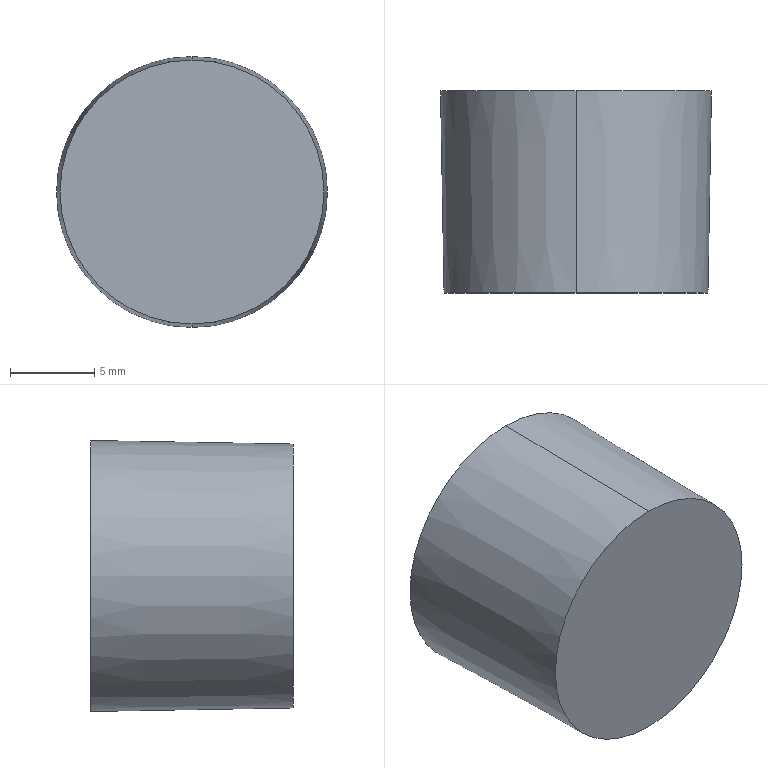Part | STEP file | 4-20.sldasm-Part-339 | 1 solid | 4 faces | box 16.088 x 12 x 16.088 mm | volume 2376 mm3 | cone 2 | plane 2
STEP:
#1=CARTESIAN_POINT('',(50.,-12.,82.165));
#2=VERTEX_POINT('',#1);
#3=CARTESIAN_POINT('',(50.,-12.,97.835));
#4=VERTEX_POINT('',#3);
#5=CARTESIAN_POINT('',(50.,-12.,90.));
#6=DIRECTION('',(0.,1.,0.));
#7=DIRECTION('',(0.,0.,-1.));
#8=AXIS2_PLACEMENT_3D('',#5,#6,#7);
#9=CIRCLE('',#8,7.835);
#10=EDGE_CURVE('',#2,#4,#9,.T.);
#11=ORIENTED_EDGE('',*,*,#10,.T.);
#12=CARTESIAN_POINT('',(50.,0.,98.044));
#13=VERTEX_POINT('',#12);
#14=CARTESIAN_POINT('',(50.,-28.035,97.555));
#15=DIRECTION('',(0.,0.9998,0.01745));
#16=VECTOR('',#15,1000.);
#17=LINE('',#14,#16);
#18=EDGE_CURVE('',#4,#13,#17,.T.);
#19=ORIENTED_EDGE('',*,*,#18,.T.);
#20=CARTESIAN_POINT('',(50.,0.,81.956));
#21=VERTEX_POINT('',#20);
#22=CARTESIAN_POINT('',(50.,0.,90.));
#23=DIRECTION('',(0.,1.,0.));
#24=DIRECTION('',(0.,0.,-1.));
#25=AXIS2_PLACEMENT_3D('',#22,#23,#24);
#26=CIRCLE('',#25,8.044);
#27=EDGE_CURVE('',#21,#13,#26,.T.);
#28=ORIENTED_EDGE('',*,*,#27,.F.);
#29=CARTESIAN_POINT('',(50.,-28.035,82.445));
#30=DIRECTION('',(0.,0.9998,-0.01745));
#31=VECTOR('',#30,1000.);
#32=LINE('',#29,#31);
#33=EDGE_CURVE('',#2,#21,#32,.T.);
#34=ORIENTED_EDGE('',*,*,#33,.F.);
#35=EDGE_LOOP('',(#11,#19,#28,#34));
#36=FACE_OUTER_BOUND('',#35,.T.);
#37=CARTESIAN_POINT('',(50.,-28.035,90.));
#38=DIRECTION('',(0.,1.,0.));
#39=DIRECTION('',(0.,0.,-1.));
#40=AXIS2_PLACEMENT_3D('',#37,#38,#39);
#41=CONICAL_SURFACE('',#40,7.555,0.01745);
#42=ADVANCED_FACE('',(#36),#41,.T.);
#43=ORIENTED_EDGE('',*,*,#10,.F.);
#44=CARTESIAN_POINT('',(50.,-12.,90.));
#45=DIRECTION('',(0.,1.,0.));
#46=DIRECTION('',(0.,0.,-1.));
#47=AXIS2_PLACEMENT_3D('',#44,#45,#46);
#48=CIRCLE('',#47,7.835);
#49=EDGE_CURVE('',#4,#2,#48,.T.);
#50=ORIENTED_EDGE('',*,*,#49,.F.);
#51=EDGE_LOOP('',(#43,#50));
#52=FACE_OUTER_BOUND('',#51,.T.);
#53=CARTESIAN_POINT('',(50.,-12.,81.956));
#54=DIRECTION('',(0.,-1.,0.));
#55=DIRECTION('',(0.,0.,1.));
#56=AXIS2_PLACEMENT_3D('',#53,#54,#55);
#57=PLANE('',#56);
#58=ADVANCED_FACE('',(#52),#57,.T.);
#59=ORIENTED_EDGE('',*,*,#18,.F.);
#60=ORIENTED_EDGE('',*,*,#49,.T.);
#61=ORIENTED_EDGE('',*,*,#33,.T.);
#62=CARTESIAN_POINT('',(50.,0.,90.));
#63=DIRECTION('',(0.,1.,0.));
#64=DIRECTION('',(0.,0.,-1.));
#65=AXIS2_PLACEMENT_3D('',#62,#63,#64);
#66=CIRCLE('',#65,8.044);
#67=EDGE_CURVE('',#13,#21,#66,.T.);
#68=ORIENTED_EDGE('',*,*,#67,.F.);
#69=EDGE_LOOP('',(#59,#60,#61,#68));
#70=FACE_OUTER_BOUND('',#69,.T.);
#71=CARTESIAN_POINT('',(50.,-28.035,90.));
#72=DIRECTION('',(0.,1.,0.));
#73=DIRECTION('',(0.,0.,-1.));
#74=AXIS2_PLACEMENT_3D('',#71,#72,#73);
#75=CONICAL_SURFACE('',#74,7.555,0.01745);
#76=ADVANCED_FACE('',(#70),#75,.T.);
#77=ORIENTED_EDGE('',*,*,#27,.T.);
#78=ORIENTED_EDGE('',*,*,#67,.T.);
#79=EDGE_LOOP('',(#77,#78));
#80=FACE_OUTER_BOUND('',#79,.T.);
#81=CARTESIAN_POINT('',(50.,0.,81.956));
#82=DIRECTION('',(0.,1.,0.));
#83=DIRECTION('',(0.,0.,-1.));
#84=AXIS2_PLACEMENT_3D('',#81,#82,#83);
#85=PLANE('',#84);
#86=ADVANCED_FACE('',(#80),#85,.T.);
#87=CLOSED_SHELL('',(#42,#58,#76,#86));
#88=MANIFOLD_SOLID_BREP('',#87);
#89=CARTESIAN_POINT('',(0.,0.,0.));
#90=DIRECTION('',(0.,0.,1.));
#91=DIRECTION('',(1.,0.,0.));
#92=AXIS2_PLACEMENT_3D('',#89,#90,#91);
#93=(LENGTH_UNIT()NAMED_UNIT(*)SI_UNIT(.MILLI.,.METRE.));
#94=UNCERTAINTY_MEASURE_WITH_UNIT(LENGTH_MEASURE(0.00001),#93,'','');
#95=(NAMED_UNIT(*)PLANE_ANGLE_UNIT()SI_UNIT($,.RADIAN.));
#96=(NAMED_UNIT(*)SI_UNIT($,.STERADIAN.)SOLID_ANGLE_UNIT());
#97=(GEOMETRIC_REPRESENTATION_CONTEXT(3)GLOBAL_UNCERTAINTY_ASSIGNED_CONTEXT((#94))GLOBAL_UNIT_ASSIGNED_CONTEXT((#93,#95,#96))REPRESENTATION_CONTEXT('',''));
#98=ADVANCED_BREP_SHAPE_REPRESENTATION('',(#88,#92),#97);